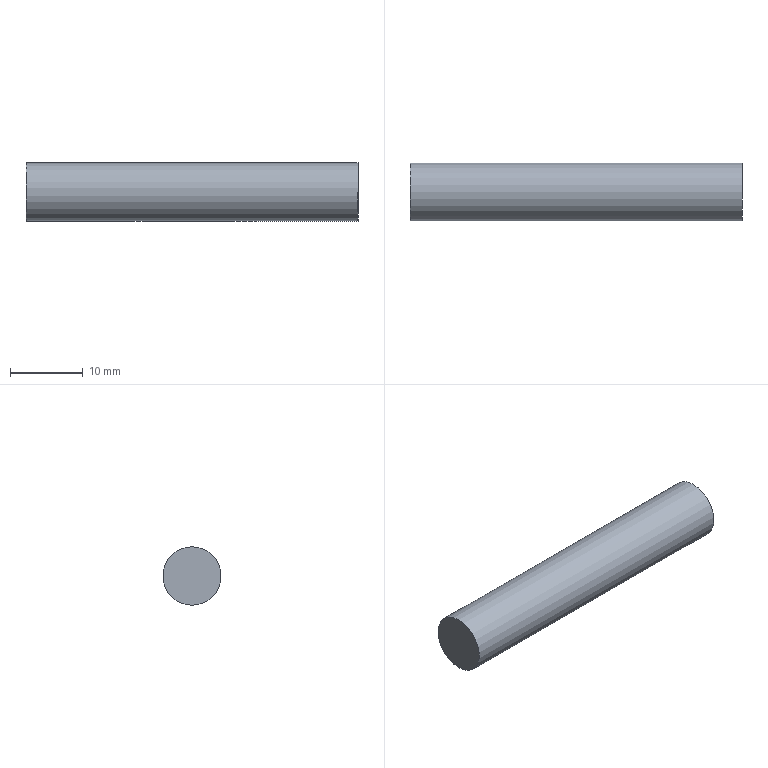Part | NX | 1 solid | 3 faces | box 45.5 x 8 x 8 mm | volume 2287 mm3 | plane 2 | cylinder 1 | commonest cylinder face diameters 8 x1
STEP:
#1=CARTESIAN_POINT('',(-22.75,0.,-4.));
#2=VERTEX_POINT('',#1);
#3=CARTESIAN_POINT('',(-22.75,0.,0.));
#4=DIRECTION('',(1.,0.,0.));
#5=DIRECTION('',(0.,0.,-1.));
#6=AXIS2_PLACEMENT_3D('',#3,#4,#5);
#7=CIRCLE('',#6,4.);
#8=EDGE_CURVE('',#2,#2,#7,.T.);
#9=ORIENTED_EDGE('',*,*,#8,.T.);
#10=EDGE_LOOP('',(#9));
#11=FACE_BOUND('',#10,.T.);
#12=CARTESIAN_POINT('',(22.75,0.,-4.));
#13=VERTEX_POINT('',#12);
#14=CARTESIAN_POINT('',(22.75,0.,0.));
#15=DIRECTION('',(1.,0.,0.));
#16=DIRECTION('',(0.,0.,-1.));
#17=AXIS2_PLACEMENT_3D('',#14,#15,#16);
#18=CIRCLE('',#17,4.);
#19=EDGE_CURVE('',#13,#13,#18,.T.);
#20=ORIENTED_EDGE('',*,*,#19,.F.);
#21=EDGE_LOOP('',(#20));
#22=FACE_BOUND('',#21,.T.);
#23=CARTESIAN_POINT('',(-22.75,0.,0.));
#24=DIRECTION('',(1.,0.,0.));
#25=DIRECTION('',(0.,0.,-1.));
#26=AXIS2_PLACEMENT_3D('',#23,#24,#25);
#27=CYLINDRICAL_SURFACE('',#26,4.);
#28=ADVANCED_FACE('',(#11,#22),#27,.T.);
#29=ORIENTED_EDGE('',*,*,#8,.F.);
#30=EDGE_LOOP('',(#29));
#31=FACE_BOUND('',#30,.T.);
#32=CARTESIAN_POINT('',(-22.75,4.,0.));
#33=DIRECTION('',(-1.,0.,0.));
#34=DIRECTION('',(0.,0.,1.));
#35=AXIS2_PLACEMENT_3D('',#32,#33,#34);
#36=PLANE('',#35);
#37=ADVANCED_FACE('',(#31),#36,.T.);
#38=ORIENTED_EDGE('',*,*,#19,.T.);
#39=EDGE_LOOP('',(#38));
#40=FACE_BOUND('',#39,.T.);
#41=CARTESIAN_POINT('',(22.75,0.,0.));
#42=DIRECTION('',(1.,0.,0.));
#43=DIRECTION('',(0.,0.,-1.));
#44=AXIS2_PLACEMENT_3D('',#41,#42,#43);
#45=PLANE('',#44);
#46=ADVANCED_FACE('',(#40),#45,.T.);
#47=CLOSED_SHELL('',(#28,#37,#46));
#48=MANIFOLD_SOLID_BREP('',#47);
#49=(LENGTH_UNIT()NAMED_UNIT(*)SI_UNIT(.MILLI.,.METRE.));
#50=UNCERTAINTY_MEASURE_WITH_UNIT(LENGTH_MEASURE(0.00001),#49,'','');
#51=(NAMED_UNIT(*)PLANE_ANGLE_UNIT()SI_UNIT($,.RADIAN.));
#52=(NAMED_UNIT(*)SI_UNIT($,.STERADIAN.)SOLID_ANGLE_UNIT());
#53=(GEOMETRIC_REPRESENTATION_CONTEXT(3)GLOBAL_UNCERTAINTY_ASSIGNED_CONTEXT((#50))GLOBAL_UNIT_ASSIGNED_CONTEXT((#49,#51,#52))REPRESENTATION_CONTEXT('',''));
#54=ADVANCED_BREP_SHAPE_REPRESENTATION('',(#48),#53);